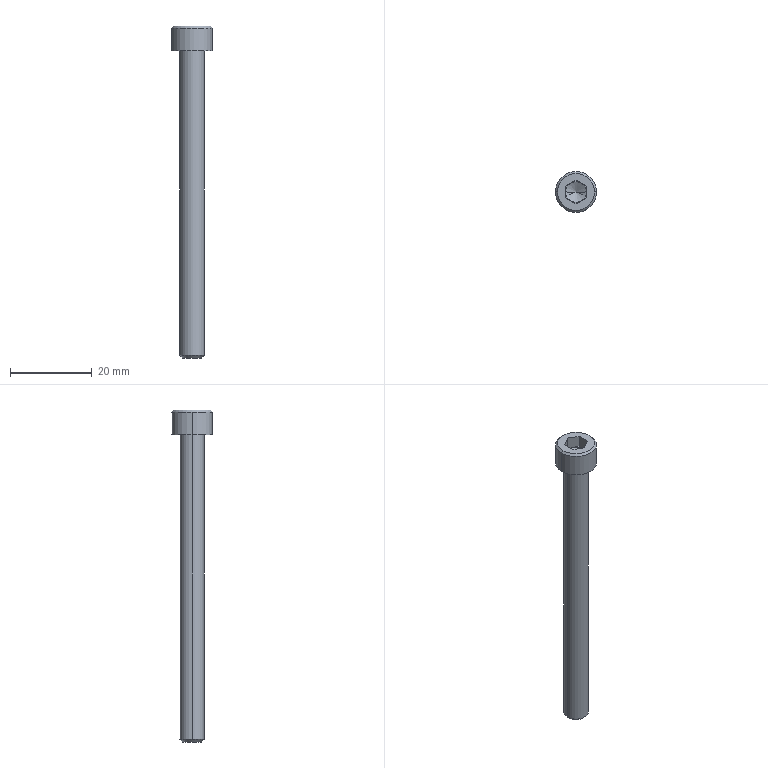Part | STEP file | 001-009-TAC01-M6-L75 | 1 solid | 25 faces | box 10 x 10 x 81 mm | volume 2510 mm3 | plane 15 | cone 6 | cylinder 4 | commonest cylinder face diameters 6 x2 10 x2